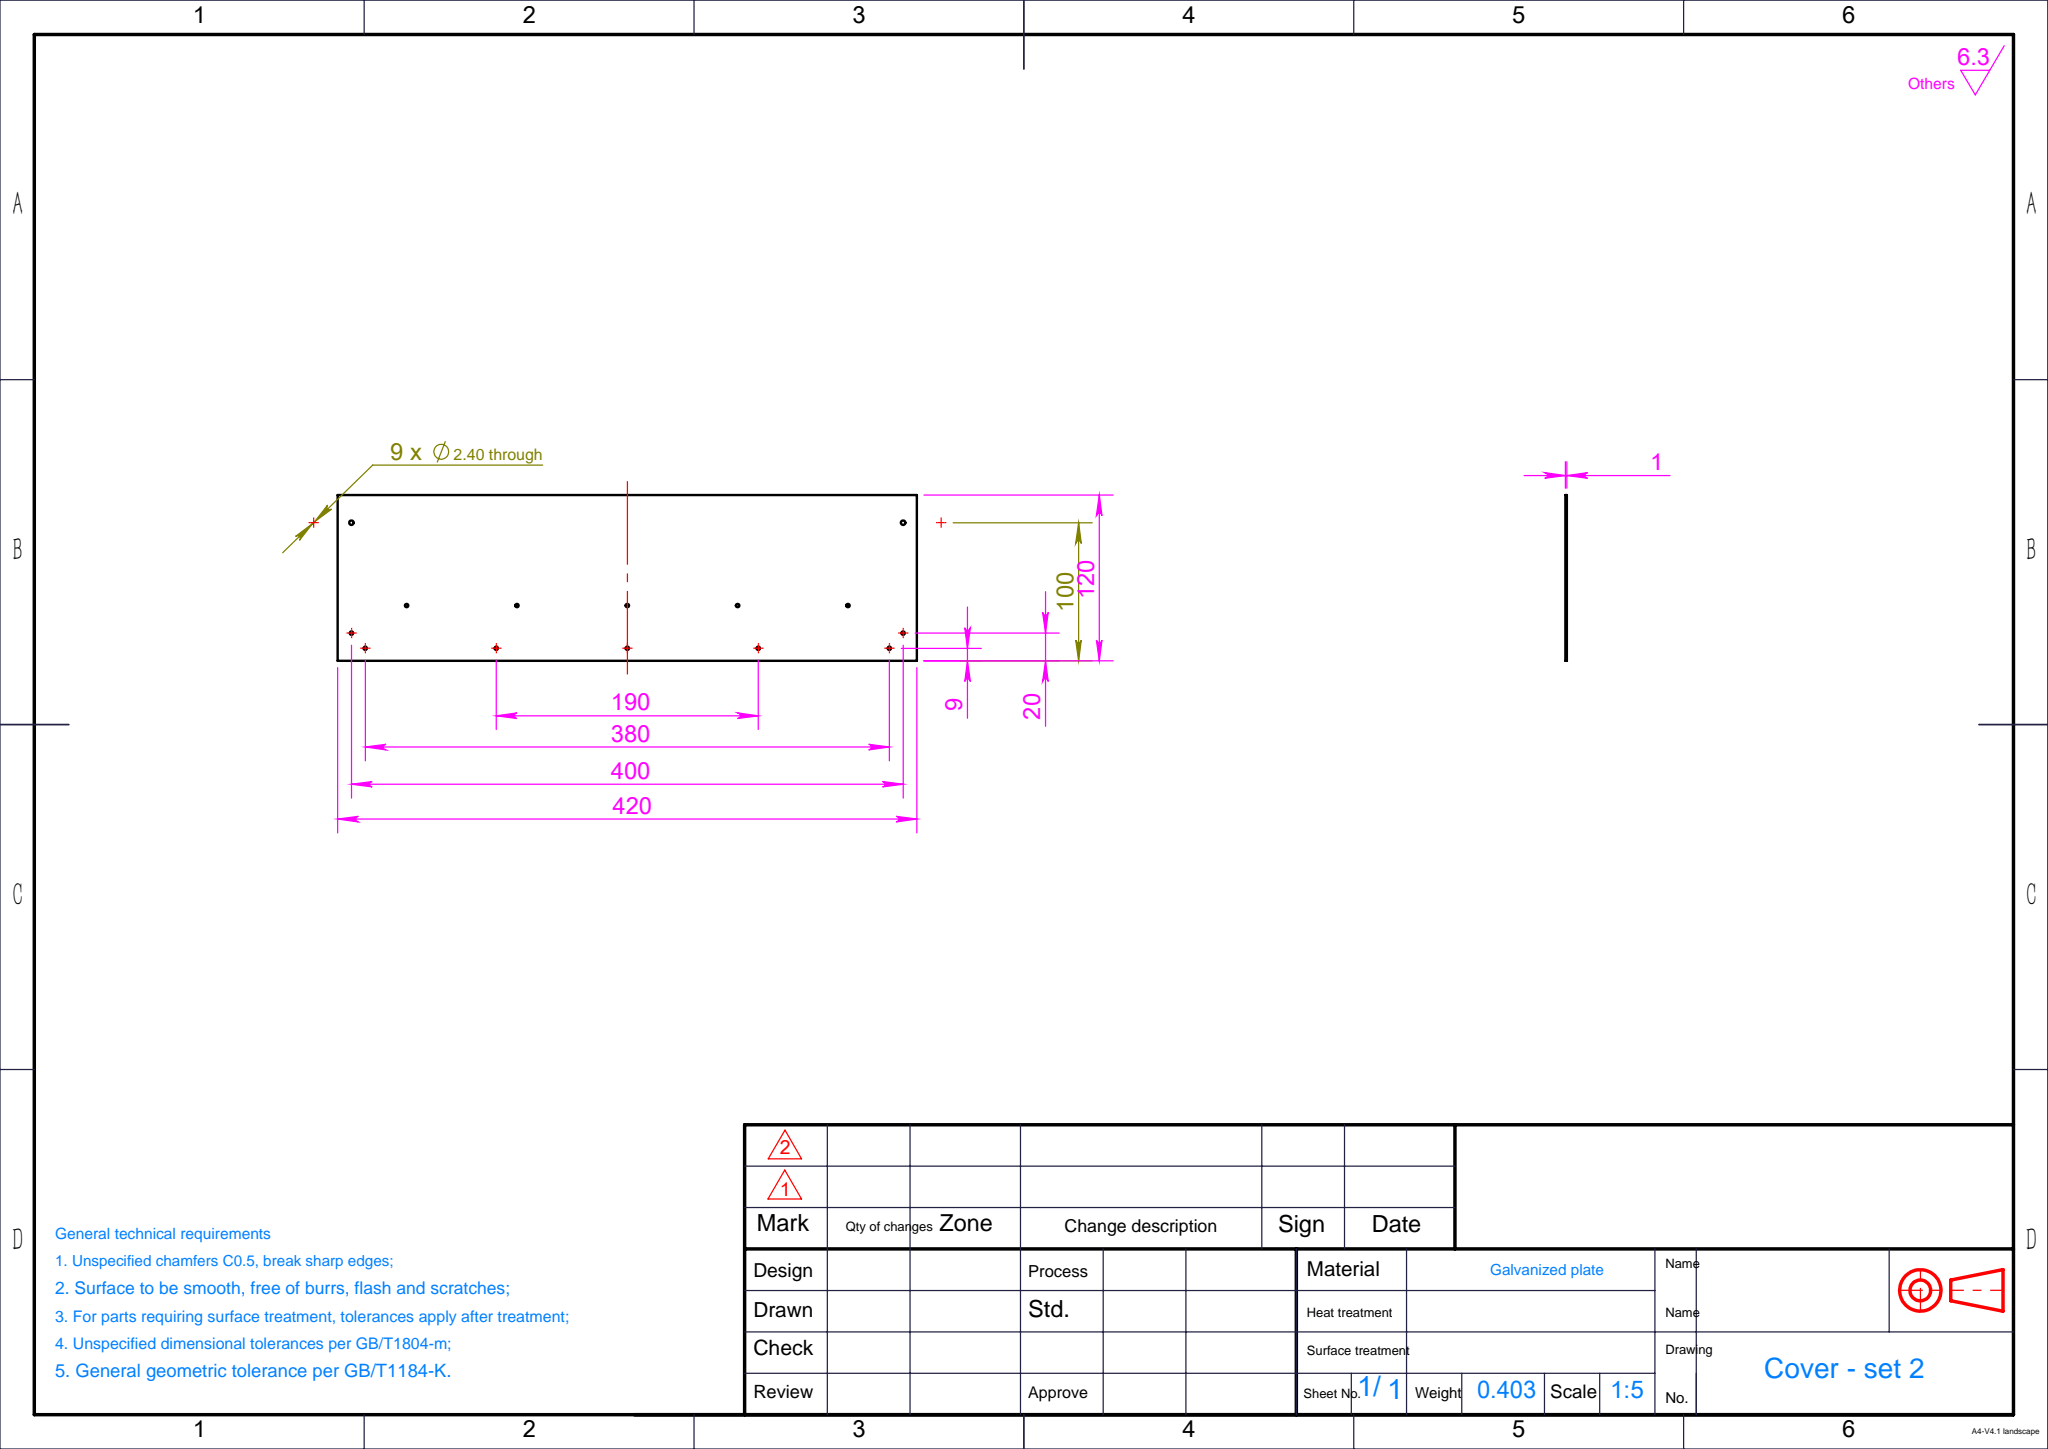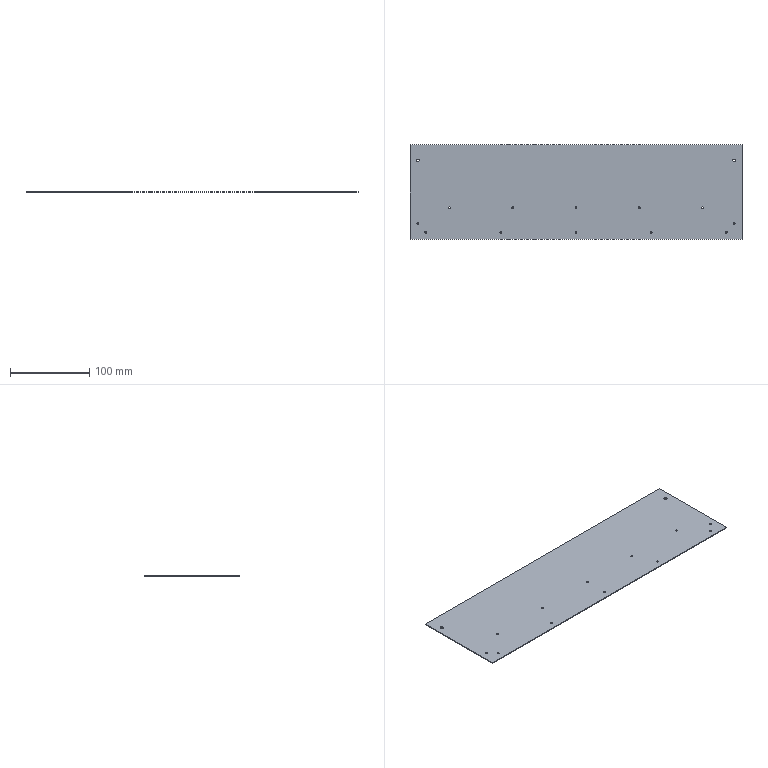Part | SolidWorks | features 3DProfileFeature 1, Chamfer 1, FlatPattern 1, HoleWzd 1, ICE 1, SMBaseFlange 1, SheetMetal 1, SketchPattern 1 | 1 solid | 38 faces | box 420 x 120 x 1 mm | volume 50324 mm3 | cylinder 28 | plane 6 | cone 4 | commonest cylinder face diameters 2.4 x24 3.2 x4